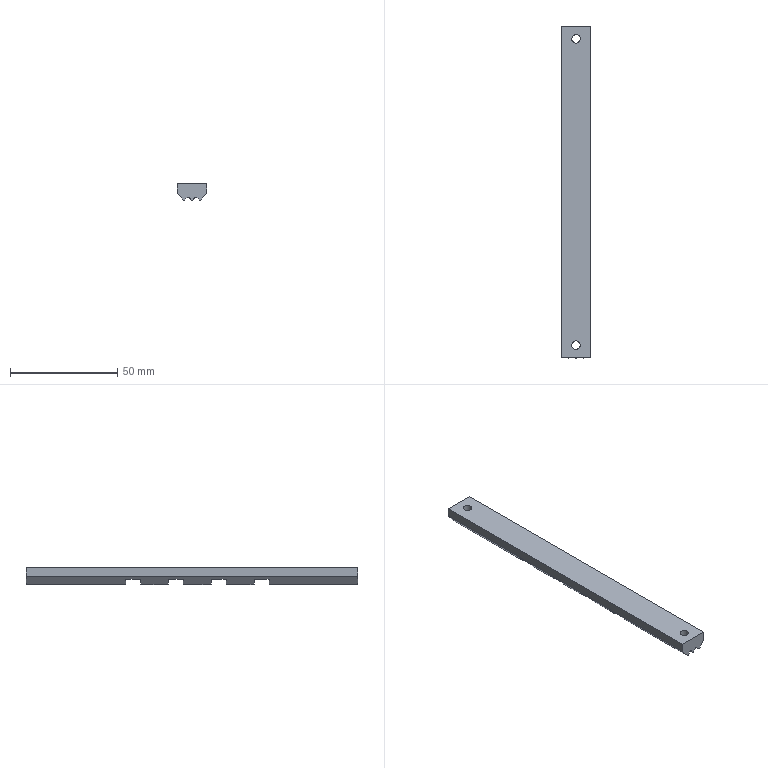Part | STEP file | 200 mesh_id1930 | 1 solid | 106 faces | box 14 x 155 x 7.945 mm | volume 13826 mm3 | plane 60 | cylinder 46 | commonest cylinder face diameters 1.04 x34 1.2 x10 4 x2